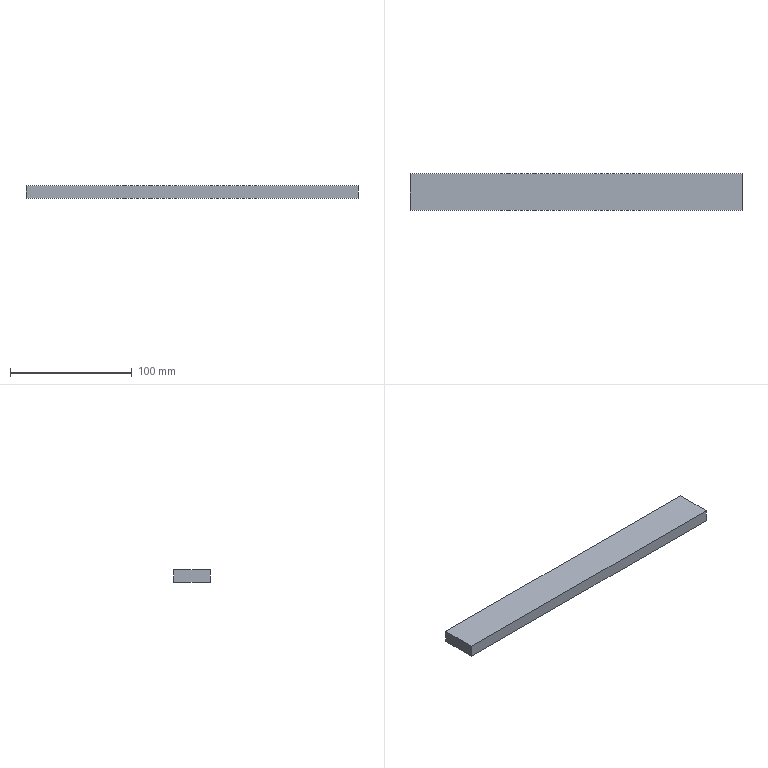Part | NX | features solid 2 | 1 solid | 6 faces | box 272.173 x 30 x 10 mm | volume 81652 mm3 | plane 6
STEP:
#1=CARTESIAN_POINT('',(212.,-140.,-15.));
#2=VERTEX_POINT('',#1);
#3=CARTESIAN_POINT('',(212.,-140.,-5.));
#4=VERTEX_POINT('',#3);
#5=CARTESIAN_POINT('',(212.,-140.,-45.));
#6=DIRECTION('',(0.,0.,-1.));
#7=VECTOR('',#6,1000.);
#8=LINE('',#5,#7);
#9=EDGE_CURVE('',#2,#4,#8,.F.);
#10=ORIENTED_EDGE('',*,*,#9,.T.);
#11=CARTESIAN_POINT('',(484.173,-140.,-5.));
#12=VERTEX_POINT('',#11);
#13=CARTESIAN_POINT('',(374.173,-140.,-5.));
#14=DIRECTION('',(1.,0.,0.));
#15=VECTOR('',#14,1000.);
#16=LINE('',#13,#15);
#17=EDGE_CURVE('',#12,#4,#16,.F.);
#18=ORIENTED_EDGE('',*,*,#17,.F.);
#19=CARTESIAN_POINT('',(484.173,-140.,-15.));
#20=VERTEX_POINT('',#19);
#21=CARTESIAN_POINT('',(484.173,-140.,-35.));
#22=DIRECTION('',(0.,0.,-1.));
#23=VECTOR('',#22,1000.);
#24=LINE('',#21,#23);
#25=EDGE_CURVE('',#20,#12,#24,.F.);
#26=ORIENTED_EDGE('',*,*,#25,.F.);
#27=CARTESIAN_POINT('',(374.173,-140.,-15.));
#28=DIRECTION('',(-1.,0.,0.));
#29=VECTOR('',#28,1000.);
#30=LINE('',#27,#29);
#31=EDGE_CURVE('',#20,#2,#30,.T.);
#32=ORIENTED_EDGE('',*,*,#31,.T.);
#33=EDGE_LOOP('',(#10,#18,#26,#32));
#34=FACE_BOUND('',#33,.T.);
#35=CARTESIAN_POINT('',(248.587,-140.,-10.));
#36=DIRECTION('',(0.,1.,0.));
#37=DIRECTION('',(0.,0.,1.));
#38=AXIS2_PLACEMENT_3D('',#35,#36,#37);
#39=PLANE('',#38);
#40=ADVANCED_FACE('',(#34),#39,.T.);
#41=CARTESIAN_POINT('',(484.173,-170.,-15.));
#42=VERTEX_POINT('',#41);
#43=CARTESIAN_POINT('',(212.,-170.,-15.));
#44=VERTEX_POINT('',#43);
#45=CARTESIAN_POINT('',(374.173,-170.,-15.));
#46=DIRECTION('',(-1.,0.,0.));
#47=VECTOR('',#46,1000.);
#48=LINE('',#45,#47);
#49=EDGE_CURVE('',#42,#44,#48,.T.);
#50=ORIENTED_EDGE('',*,*,#49,.F.);
#51=CARTESIAN_POINT('',(484.173,-170.,-5.));
#52=VERTEX_POINT('',#51);
#53=CARTESIAN_POINT('',(484.173,-170.,-35.));
#54=DIRECTION('',(0.,0.,-1.));
#55=VECTOR('',#54,1000.);
#56=LINE('',#53,#55);
#57=EDGE_CURVE('',#42,#52,#56,.F.);
#58=ORIENTED_EDGE('',*,*,#57,.T.);
#59=CARTESIAN_POINT('',(212.,-170.,-5.));
#60=VERTEX_POINT('',#59);
#61=CARTESIAN_POINT('',(374.173,-170.,-5.));
#62=DIRECTION('',(1.,0.,0.));
#63=VECTOR('',#62,1000.);
#64=LINE('',#61,#63);
#65=EDGE_CURVE('',#52,#60,#64,.F.);
#66=ORIENTED_EDGE('',*,*,#65,.T.);
#67=CARTESIAN_POINT('',(212.,-170.,-45.));
#68=DIRECTION('',(0.,0.,-1.));
#69=VECTOR('',#68,1000.);
#70=LINE('',#67,#69);
#71=EDGE_CURVE('',#44,#60,#70,.F.);
#72=ORIENTED_EDGE('',*,*,#71,.F.);
#73=EDGE_LOOP('',(#50,#58,#66,#72));
#74=FACE_BOUND('',#73,.T.);
#75=CARTESIAN_POINT('',(374.173,-170.,-35.));
#76=DIRECTION('',(0.,-1.,0.));
#77=DIRECTION('',(0.,0.,-1.));
#78=AXIS2_PLACEMENT_3D('',#75,#76,#77);
#79=PLANE('',#78);
#80=ADVANCED_FACE('',(#74),#79,.T.);
#81=ORIENTED_EDGE('',*,*,#25,.T.);
#82=CARTESIAN_POINT('',(484.173,-140.,-5.));
#83=DIRECTION('',(0.,-1.,0.));
#84=VECTOR('',#83,1000.);
#85=LINE('',#82,#84);
#86=EDGE_CURVE('',#12,#52,#85,.T.);
#87=ORIENTED_EDGE('',*,*,#86,.T.);
#88=ORIENTED_EDGE('',*,*,#57,.F.);
#89=CARTESIAN_POINT('',(484.173,-140.,-15.));
#90=DIRECTION('',(0.,1.,0.));
#91=VECTOR('',#90,1000.);
#92=LINE('',#89,#91);
#93=EDGE_CURVE('',#20,#42,#92,.F.);
#94=ORIENTED_EDGE('',*,*,#93,.F.);
#95=EDGE_LOOP('',(#81,#87,#88,#94));
#96=FACE_BOUND('',#95,.T.);
#97=CARTESIAN_POINT('',(484.173,-140.,-35.));
#98=DIRECTION('',(-1.,0.,0.));
#99=DIRECTION('',(0.,0.,1.));
#100=AXIS2_PLACEMENT_3D('',#97,#98,#99);
#101=PLANE('',#100);
#102=ADVANCED_FACE('',(#96),#101,.F.);
#103=CARTESIAN_POINT('',(212.,-170.,-15.));
#104=DIRECTION('',(0.,1.,0.));
#105=VECTOR('',#104,1000.);
#106=LINE('',#103,#105);
#107=EDGE_CURVE('',#2,#44,#106,.F.);
#108=ORIENTED_EDGE('',*,*,#107,.T.);
#109=ORIENTED_EDGE('',*,*,#71,.T.);
#110=CARTESIAN_POINT('',(212.,-170.,-5.));
#111=DIRECTION('',(0.,1.,0.));
#112=VECTOR('',#111,1000.);
#113=LINE('',#110,#112);
#114=EDGE_CURVE('',#4,#60,#113,.F.);
#115=ORIENTED_EDGE('',*,*,#114,.F.);
#116=ORIENTED_EDGE('',*,*,#9,.F.);
#117=EDGE_LOOP('',(#108,#109,#115,#116));
#118=FACE_BOUND('',#117,.T.);
#119=CARTESIAN_POINT('',(212.,-170.,-10.));
#120=DIRECTION('',(1.,0.,0.));
#121=DIRECTION('',(0.,0.,-1.));
#122=AXIS2_PLACEMENT_3D('',#119,#120,#121);
#123=PLANE('',#122);
#124=ADVANCED_FACE('',(#118),#123,.F.);
#125=ORIENTED_EDGE('',*,*,#17,.T.);
#126=ORIENTED_EDGE('',*,*,#114,.T.);
#127=ORIENTED_EDGE('',*,*,#65,.F.);
#128=ORIENTED_EDGE('',*,*,#86,.F.);
#129=EDGE_LOOP('',(#125,#126,#127,#128));
#130=FACE_BOUND('',#129,.T.);
#131=CARTESIAN_POINT('',(374.173,-140.,-5.));
#132=DIRECTION('',(0.,0.,-1.));
#133=DIRECTION('',(-1.,0.,0.));
#134=AXIS2_PLACEMENT_3D('',#131,#132,#133);
#135=PLANE('',#134);
#136=ADVANCED_FACE('',(#130),#135,.F.);
#137=ORIENTED_EDGE('',*,*,#31,.F.);
#138=ORIENTED_EDGE('',*,*,#93,.T.);
#139=ORIENTED_EDGE('',*,*,#49,.T.);
#140=ORIENTED_EDGE('',*,*,#107,.F.);
#141=EDGE_LOOP('',(#137,#138,#139,#140));
#142=FACE_BOUND('',#141,.T.);
#143=CARTESIAN_POINT('',(374.173,-140.,-15.));
#144=DIRECTION('',(0.,0.,-1.));
#145=DIRECTION('',(-1.,0.,0.));
#146=AXIS2_PLACEMENT_3D('',#143,#144,#145);
#147=PLANE('',#146);
#148=ADVANCED_FACE('',(#142),#147,.T.);
#149=CLOSED_SHELL('',(#40,#80,#102,#124,#136,#148));
#150=MANIFOLD_SOLID_BREP('',#149);
#151=(LENGTH_UNIT()NAMED_UNIT(*)SI_UNIT(.MILLI.,.METRE.));
#152=UNCERTAINTY_MEASURE_WITH_UNIT(LENGTH_MEASURE(0.00001),#151,'','');
#153=(NAMED_UNIT(*)PLANE_ANGLE_UNIT()SI_UNIT($,.RADIAN.));
#154=(NAMED_UNIT(*)SI_UNIT($,.STERADIAN.)SOLID_ANGLE_UNIT());
#155=(GEOMETRIC_REPRESENTATION_CONTEXT(3)GLOBAL_UNCERTAINTY_ASSIGNED_CONTEXT((#152))GLOBAL_UNIT_ASSIGNED_CONTEXT((#151,#153,#154))REPRESENTATION_CONTEXT('',''));
#156=ADVANCED_BREP_SHAPE_REPRESENTATION('',(#150),#155);